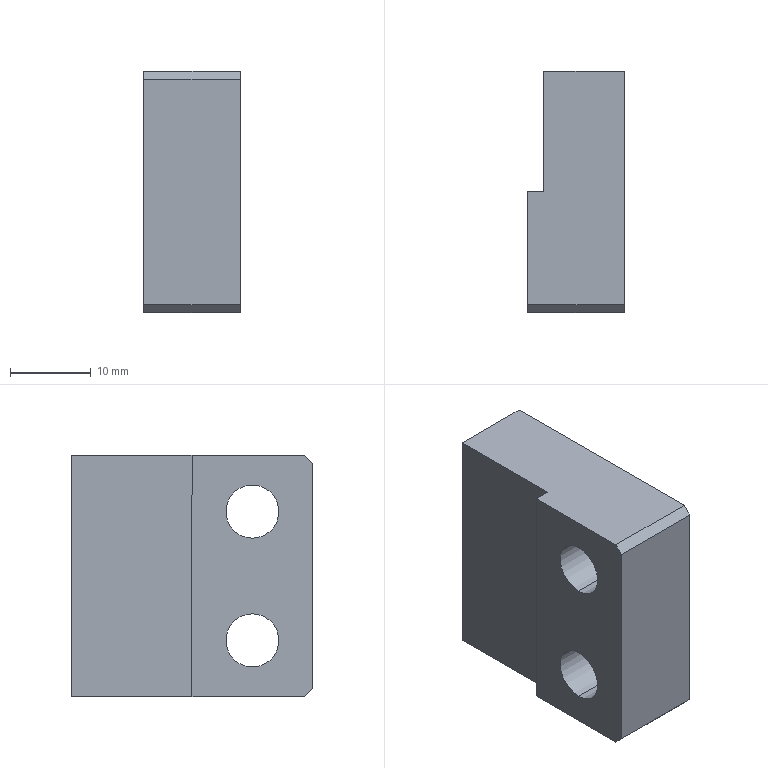Part | STEP file | M-05-006A_default | 1 solid | 20 faces | box 12 x 30 x 30 mm | volume 8337 mm3 | plane 12 | cylinder 8 | commonest cylinder face diameters 6.6 x4 11 x4
STEP:
#1=CARTESIAN_POINT('',(0.,0.,0.));
#2=DIRECTION('',(0.,0.,1.));
#3=DIRECTION('',(1.,0.,0.));
#4=AXIS2_PLACEMENT_3D('',#1,#2,#3);
#5=CARTESIAN_POINT('',(6.2,-7.5,4.7));
#6=VERTEX_POINT('',#5);
#7=CARTESIAN_POINT('',(12.2,-7.5,4.7));
#8=VERTEX_POINT('',#7);
#9=CARTESIAN_POINT('',(18.2,-7.5,4.7));
#10=DIRECTION('',(1.,0.,0.));
#11=VECTOR('',#10,1.);
#12=LINE('',#9,#11);
#13=CARTESIAN_POINT('',(18.2,-7.5,8.));
#14=DIRECTION('',(1.,0.,0.));
#15=DIRECTION('',(0.,0.,-1.));
#16=AXIS2_PLACEMENT_3D('',#13,#14,#15);
#17=CYLINDRICAL_SURFACE('',#16,3.3);
#18=CARTESIAN_POINT('',(6.283,0.));
#19=DIRECTION('',(0.,1.));
#20=VECTOR('',#19,1.);
#21=LINE('',#18,#20);
#22=(GEOMETRIC_REPRESENTATION_CONTEXT(2)PARAMETRIC_REPRESENTATION_CONTEXT()REPRESENTATION_CONTEXT('',''));
#23=DEFINITIONAL_REPRESENTATION('',(#21),#22);
#24=PCURVE('',#17,#23);
#25=CARTESIAN_POINT('',(18.2,-7.5,8.));
#26=DIRECTION('',(1.,0.,0.));
#27=DIRECTION('',(0.,0.,-1.));
#28=AXIS2_PLACEMENT_3D('',#25,#26,#27);
#29=CYLINDRICAL_SURFACE('',#28,3.3);
#30=CARTESIAN_POINT('',(0.,0.));
#31=DIRECTION('',(0.,1.));
#32=VECTOR('',#31,1.);
#33=LINE('',#30,#32);
#34=(GEOMETRIC_REPRESENTATION_CONTEXT(2)PARAMETRIC_REPRESENTATION_CONTEXT()REPRESENTATION_CONTEXT('',''));
#35=DEFINITIONAL_REPRESENTATION('',(#33),#34);
#36=PCURVE('',#29,#35);
#37=SURFACE_CURVE('',#12,(#24,#36),.PCURVE_S1.);
#38=EDGE_CURVE('',#6,#8,#37,.T.);
#39=ORIENTED_EDGE('',*,*,#38,.T.);
#40=CARTESIAN_POINT('',(12.2,-7.5,11.3));
#41=VERTEX_POINT('',#40);
#42=CARTESIAN_POINT('',(12.2,-7.5,8.));
#43=DIRECTION('',(1.,0.,0.));
#44=DIRECTION('',(0.,0.,-1.));
#45=AXIS2_PLACEMENT_3D('',#42,#43,#44);
#46=CIRCLE('',#45,3.3);
#47=CARTESIAN_POINT('',(0.,-6.));
#48=DIRECTION('',(1.,0.));
#49=VECTOR('',#48,1.);
#50=LINE('',#47,#49);
#51=(GEOMETRIC_REPRESENTATION_CONTEXT(2)PARAMETRIC_REPRESENTATION_CONTEXT()REPRESENTATION_CONTEXT('',''));
#52=DEFINITIONAL_REPRESENTATION('',(#50),#51);
#53=PCURVE('',#17,#52);
#54=CARTESIAN_POINT('',(12.2,-4.2,8.));
#55=DIRECTION('',(-1.,0.,0.));
#56=DIRECTION('',(0.,0.,1.));
#57=AXIS2_PLACEMENT_3D('',#54,#55,#56);
#58=PLANE('',#57);
#59=CARTESIAN_POINT('',(-3.3,-3.3));
#60=CARTESIAN_POINT('',(-3.3,2.416));
#61=CARTESIAN_POINT('',(1.65,-0.4421));
#62=CARTESIAN_POINT('',(6.6,-3.3));
#63=CARTESIAN_POINT('',(1.65,-6.158));
#64=CARTESIAN_POINT('',(-3.3,-9.016));
#65=CARTESIAN_POINT('',(-3.3,-3.3));
#66=(BOUNDED_CURVE()B_SPLINE_CURVE(2,(#59,#60,#61,#62,#63,#64,#65),.UNSPECIFIED.,.T.,.F.)B_SPLINE_CURVE_WITH_KNOTS((1,2,2,2,2,1),(-2.094,0.,2.094,4.189,6.283,8.378),.UNSPECIFIED.)CURVE()GEOMETRIC_REPRESENTATION_ITEM()RATIONAL_B_SPLINE_CURVE((1.,0.5,1.,0.5,1.,0.5,1.))REPRESENTATION_ITEM(''));
#67=(GEOMETRIC_REPRESENTATION_CONTEXT(2)PARAMETRIC_REPRESENTATION_CONTEXT()REPRESENTATION_CONTEXT('',''));
#68=DEFINITIONAL_REPRESENTATION('',(#66),#67);
#69=PCURVE('',#58,#68);
#70=SURFACE_CURVE('',#46,(#53,#69),.PCURVE_S1.);
#71=EDGE_CURVE('',#41,#8,#70,.T.);
#72=ORIENTED_EDGE('',*,*,#71,.F.);
#73=CARTESIAN_POINT('',(6.2,-7.5,11.3));
#74=VERTEX_POINT('',#73);
#75=CARTESIAN_POINT('',(18.2,-7.5,11.3));
#76=DIRECTION('',(1.,0.,0.));
#77=VECTOR('',#76,1.);
#78=LINE('',#75,#77);
#79=CARTESIAN_POINT('',(3.142,0.));
#80=DIRECTION('',(0.,1.));
#81=VECTOR('',#80,1.);
#82=LINE('',#79,#81);
#83=(GEOMETRIC_REPRESENTATION_CONTEXT(2)PARAMETRIC_REPRESENTATION_CONTEXT()REPRESENTATION_CONTEXT('',''));
#84=DEFINITIONAL_REPRESENTATION('',(#82),#83);
#85=PCURVE('',#17,#84);
#86=CARTESIAN_POINT('',(3.142,0.));
#87=DIRECTION('',(0.,1.));
#88=VECTOR('',#87,1.);
#89=LINE('',#86,#88);
#90=(GEOMETRIC_REPRESENTATION_CONTEXT(2)PARAMETRIC_REPRESENTATION_CONTEXT()REPRESENTATION_CONTEXT('',''));
#91=DEFINITIONAL_REPRESENTATION('',(#89),#90);
#92=PCURVE('',#29,#91);
#93=SURFACE_CURVE('',#78,(#85,#92),.PCURVE_S1.);
#94=EDGE_CURVE('',#74,#41,#93,.T.);
#95=ORIENTED_EDGE('',*,*,#94,.F.);
#96=CARTESIAN_POINT('',(6.2,-7.5,8.));
#97=DIRECTION('',(1.,0.,0.));
#98=DIRECTION('',(0.,0.,-1.));
#99=AXIS2_PLACEMENT_3D('',#96,#97,#98);
#100=CIRCLE('',#99,3.3);
#101=CARTESIAN_POINT('',(0.,-12.));
#102=DIRECTION('',(1.,0.));
#103=VECTOR('',#102,1.);
#104=LINE('',#101,#103);
#105=(GEOMETRIC_REPRESENTATION_CONTEXT(2)PARAMETRIC_REPRESENTATION_CONTEXT()REPRESENTATION_CONTEXT('',''));
#106=DEFINITIONAL_REPRESENTATION('',(#104),#105);
#107=PCURVE('',#17,#106);
#108=CARTESIAN_POINT('',(6.2,15.,15.));
#109=DIRECTION('',(1.,0.,0.));
#110=DIRECTION('',(0.,0.,-1.));
#111=AXIS2_PLACEMENT_3D('',#108,#109,#110);
#112=PLANE('',#111);
#113=CARTESIAN_POINT('',(7.,-22.5));
#114=DIRECTION('',(1.,0.));
#115=AXIS2_PLACEMENT_2D('',#113,#114);
#116=CIRCLE('',#115,3.3);
#117=(GEOMETRIC_REPRESENTATION_CONTEXT(2)PARAMETRIC_REPRESENTATION_CONTEXT()REPRESENTATION_CONTEXT('',''));
#118=DEFINITIONAL_REPRESENTATION('',(#116),#117);
#119=PCURVE('',#112,#118);
#120=SURFACE_CURVE('',#100,(#107,#119),.PCURVE_S1.);
#121=EDGE_CURVE('',#74,#6,#120,.T.);
#122=ORIENTED_EDGE('',*,*,#121,.T.);
#123=EDGE_LOOP('',(#39,#72,#95,#122));
#124=FACE_BOUND('',#123,.F.);
#125=ADVANCED_FACE('',(#124),#17,.F.);
#126=CARTESIAN_POINT('',(12.2,-7.5,2.5));
#127=VERTEX_POINT('',#126);
#128=CARTESIAN_POINT('',(18.2,-7.5,2.5));
#129=VERTEX_POINT('',#128);
#130=CARTESIAN_POINT('',(18.2,-7.5,2.5));
#131=DIRECTION('',(1.,0.,0.));
#132=VECTOR('',#131,1.);
#133=LINE('',#130,#132);
#134=CARTESIAN_POINT('',(18.2,-7.5,8.));
#135=DIRECTION('',(1.,0.,0.));
#136=DIRECTION('',(0.,0.,-1.));
#137=AXIS2_PLACEMENT_3D('',#134,#135,#136);
#138=CYLINDRICAL_SURFACE('',#137,5.5);
#139=CARTESIAN_POINT('',(6.283,0.));
#140=DIRECTION('',(0.,1.));
#141=VECTOR('',#140,1.);
#142=LINE('',#139,#141);
#143=(GEOMETRIC_REPRESENTATION_CONTEXT(2)PARAMETRIC_REPRESENTATION_CONTEXT()REPRESENTATION_CONTEXT('',''));
#144=DEFINITIONAL_REPRESENTATION('',(#142),#143);
#145=PCURVE('',#138,#144);
#146=CARTESIAN_POINT('',(18.2,-7.5,8.));
#147=DIRECTION('',(1.,0.,0.));
#148=DIRECTION('',(0.,0.,-1.));
#149=AXIS2_PLACEMENT_3D('',#146,#147,#148);
#150=CYLINDRICAL_SURFACE('',#149,5.5);
#151=CARTESIAN_POINT('',(0.,0.));
#152=DIRECTION('',(0.,1.));
#153=VECTOR('',#152,1.);
#154=LINE('',#151,#153);
#155=(GEOMETRIC_REPRESENTATION_CONTEXT(2)PARAMETRIC_REPRESENTATION_CONTEXT()REPRESENTATION_CONTEXT('',''));
#156=DEFINITIONAL_REPRESENTATION('',(#154),#155);
#157=PCURVE('',#150,#156);
#158=SURFACE_CURVE('',#133,(#145,#157),.PCURVE_S1.);
#159=EDGE_CURVE('',#127,#129,#158,.T.);
#160=ORIENTED_EDGE('',*,*,#159,.T.);
#161=CARTESIAN_POINT('',(18.2,-7.5,13.5));
#162=VERTEX_POINT('',#161);
#163=CARTESIAN_POINT('',(18.2,-7.5,8.));
#164=DIRECTION('',(1.,0.,0.));
#165=DIRECTION('',(0.,0.,-1.));
#166=AXIS2_PLACEMENT_3D('',#163,#164,#165);
#167=CIRCLE('',#166,5.5);
#168=CARTESIAN_POINT('',(0.,0.));
#169=DIRECTION('',(1.,0.));
#170=VECTOR('',#169,1.);
#171=LINE('',#168,#170);
#172=(GEOMETRIC_REPRESENTATION_CONTEXT(2)PARAMETRIC_REPRESENTATION_CONTEXT()REPRESENTATION_CONTEXT('',''));
#173=DEFINITIONAL_REPRESENTATION('',(#171),#172);
#174=PCURVE('',#138,#173);
#175=CARTESIAN_POINT('',(18.2,15.,15.));
#176=DIRECTION('',(-1.,0.,0.));
#177=DIRECTION('',(0.,0.,1.));
#178=AXIS2_PLACEMENT_3D('',#175,#176,#177);
#179=PLANE('',#178);
#180=CARTESIAN_POINT('',(-12.5,-22.5));
#181=CARTESIAN_POINT('',(-12.5,-12.974));
#182=CARTESIAN_POINT('',(-4.25,-17.737));
#183=CARTESIAN_POINT('',(4.,-22.5));
#184=CARTESIAN_POINT('',(-4.25,-27.263));
#185=CARTESIAN_POINT('',(-12.5,-32.026));
#186=CARTESIAN_POINT('',(-12.5,-22.5));
#187=(BOUNDED_CURVE()B_SPLINE_CURVE(2,(#180,#181,#182,#183,#184,#185,#186),.UNSPECIFIED.,.T.,.F.)B_SPLINE_CURVE_WITH_KNOTS((1,2,2,2,2,1),(-2.094,0.,2.094,4.189,6.283,8.378),.UNSPECIFIED.)CURVE()GEOMETRIC_REPRESENTATION_ITEM()RATIONAL_B_SPLINE_CURVE((1.,0.5,1.,0.5,1.,0.5,1.))REPRESENTATION_ITEM(''));
#188=(GEOMETRIC_REPRESENTATION_CONTEXT(2)PARAMETRIC_REPRESENTATION_CONTEXT()REPRESENTATION_CONTEXT('',''));
#189=DEFINITIONAL_REPRESENTATION('',(#187),#188);
#190=PCURVE('',#179,#189);
#191=SURFACE_CURVE('',#167,(#174,#190),.PCURVE_S1.);
#192=EDGE_CURVE('',#162,#129,#191,.T.);
#193=ORIENTED_EDGE('',*,*,#192,.F.);
#194=CARTESIAN_POINT('',(12.2,-7.5,13.5));
#195=VERTEX_POINT('',#194);
#196=CARTESIAN_POINT('',(18.2,-7.5,13.5));
#197=DIRECTION('',(1.,0.,0.));
#198=VECTOR('',#197,1.);
#199=LINE('',#196,#198);
#200=CARTESIAN_POINT('',(3.142,0.));
#201=DIRECTION('',(0.,1.));
#202=VECTOR('',#201,1.);
#203=LINE('',#200,#202);
#204=(GEOMETRIC_REPRESENTATION_CONTEXT(2)PARAMETRIC_REPRESENTATION_CONTEXT()REPRESENTATION_CONTEXT('',''));
#205=DEFINITIONAL_REPRESENTATION('',(#203),#204);
#206=PCURVE('',#138,#205);
#207=CARTESIAN_POINT('',(3.142,0.));
#208=DIRECTION('',(0.,1.));
#209=VECTOR('',#208,1.);
#210=LINE('',#207,#209);
#211=(GEOMETRIC_REPRESENTATION_CONTEXT(2)PARAMETRIC_REPRESENTATION_CONTEXT()REPRESENTATION_CONTEXT('',''));
#212=DEFINITIONAL_REPRESENTATION('',(#210),#211);
#213=PCURVE('',#150,#212);
#214=SURFACE_CURVE('',#199,(#206,#213),.PCURVE_S1.);
#215=EDGE_CURVE('',#195,#162,#214,.T.);
#216=ORIENTED_EDGE('',*,*,#215,.F.);
#217=CARTESIAN_POINT('',(12.2,-7.5,8.));
#218=DIRECTION('',(1.,0.,0.));
#219=DIRECTION('',(0.,0.,-1.));
#220=AXIS2_PLACEMENT_3D('',#217,#218,#219);
#221=CIRCLE('',#220,5.5);
#222=CARTESIAN_POINT('',(0.,-6.));
#223=DIRECTION('',(1.,0.));
#224=VECTOR('',#223,1.);
#225=LINE('',#222,#224);
#226=(GEOMETRIC_REPRESENTATION_CONTEXT(2)PARAMETRIC_REPRESENTATION_CONTEXT()REPRESENTATION_CONTEXT('',''));
#227=DEFINITIONAL_REPRESENTATION('',(#225),#226);
#228=PCURVE('',#138,#227);
#229=CARTESIAN_POINT('',(-5.5,-3.3));
#230=CARTESIAN_POINT('',(-5.5,6.226));
#231=CARTESIAN_POINT('',(2.75,1.463));
#232=CARTESIAN_POINT('',(11.,-3.3));
#233=CARTESIAN_POINT('',(2.75,-8.063));
#234=CARTESIAN_POINT('',(-5.5,-12.826));
#235=CARTESIAN_POINT('',(-5.5,-3.3));
#236=(BOUNDED_CURVE()B_SPLINE_CURVE(2,(#229,#230,#231,#232,#233,#234,#235),.UNSPECIFIED.,.T.,.F.)B_SPLINE_CURVE_WITH_KNOTS((1,2,2,2,2,1),(-2.094,0.,2.094,4.189,6.283,8.378),.UNSPECIFIED.)CURVE()GEOMETRIC_REPRESENTATION_ITEM()RATIONAL_B_SPLINE_CURVE((1.,0.5,1.,0.5,1.,0.5,1.))REPRESENTATION_ITEM(''));
#237=(GEOMETRIC_REPRESENTATION_CONTEXT(2)PARAMETRIC_REPRESENTATION_CONTEXT()REPRESENTATION_CONTEXT('',''));
#238=DEFINITIONAL_REPRESENTATION('',(#236),#237);
#239=PCURVE('',#58,#238);
#240=SURFACE_CURVE('',#221,(#228,#239),.PCURVE_S1.);
#241=EDGE_CURVE('',#195,#127,#240,.T.);
#242=ORIENTED_EDGE('',*,*,#241,.T.);
#243=EDGE_LOOP('',(#160,#193,#216,#242));
#244=FACE_BOUND('',#243,.F.);
#245=ADVANCED_FACE('',(#244),#138,.F.);
#246=CARTESIAN_POINT('',(6.2,-7.5,-11.3));
#247=VERTEX_POINT('',#246);
#248=CARTESIAN_POINT('',(12.2,-7.5,-11.3));
#249=VERTEX_POINT('',#248);
#250=CARTESIAN_POINT('',(18.2,-7.5,-11.3));
#251=DIRECTION('',(1.,0.,0.));
#252=VECTOR('',#251,1.);
#253=LINE('',#250,#252);
#254=CARTESIAN_POINT('',(18.2,-7.5,-8.));
#255=DIRECTION('',(1.,0.,0.));
#256=DIRECTION('',(0.,0.,-1.));
#257=AXIS2_PLACEMENT_3D('',#254,#255,#256);
#258=CYLINDRICAL_SURFACE('',#257,3.3);
#259=CARTESIAN_POINT('',(6.283,0.));
#260=DIRECTION('',(0.,1.));
#261=VECTOR('',#260,1.);
#262=LINE('',#259,#261);
#263=(GEOMETRIC_REPRESENTATION_CONTEXT(2)PARAMETRIC_REPRESENTATION_CONTEXT()REPRESENTATION_CONTEXT('',''));
#264=DEFINITIONAL_REPRESENTATION('',(#262),#263);
#265=PCURVE('',#258,#264);
#266=CARTESIAN_POINT('',(18.2,-7.5,-8.));
#267=DIRECTION('',(1.,0.,0.));
#268=DIRECTION('',(0.,0.,-1.));
#269=AXIS2_PLACEMENT_3D('',#266,#267,#268);
#270=CYLINDRICAL_SURFACE('',#269,3.3);
#271=CARTESIAN_POINT('',(0.,0.));
#272=DIRECTION('',(0.,1.));
#273=VECTOR('',#272,1.);
#274=LINE('',#271,#273);
#275=(GEOMETRIC_REPRESENTATION_CONTEXT(2)PARAMETRIC_REPRESENTATION_CONTEXT()REPRESENTATION_CONTEXT('',''));
#276=DEFINITIONAL_REPRESENTATION('',(#274),#275);
#277=PCURVE('',#270,#276);
#278=SURFACE_CURVE('',#253,(#265,#277),.PCURVE_S1.);
#279=EDGE_CURVE('',#247,#249,#278,.T.);
#280=ORIENTED_EDGE('',*,*,#279,.T.);
#281=CARTESIAN_POINT('',(12.2,-7.5,-4.7));
#282=VERTEX_POINT('',#281);
#283=CARTESIAN_POINT('',(12.2,-7.5,-8.));
#284=DIRECTION('',(1.,0.,0.));
#285=DIRECTION('',(0.,0.,-1.));
#286=AXIS2_PLACEMENT_3D('',#283,#284,#285);
#287=CIRCLE('',#286,3.3);
#288=CARTESIAN_POINT('',(0.,-6.));
#289=DIRECTION('',(1.,0.));
#290=VECTOR('',#289,1.);
#291=LINE('',#288,#290);
#292=(GEOMETRIC_REPRESENTATION_CONTEXT(2)PARAMETRIC_REPRESENTATION_CONTEXT()REPRESENTATION_CONTEXT('',''));
#293=DEFINITIONAL_REPRESENTATION('',(#291),#292);
#294=PCURVE('',#258,#293);
#295=CARTESIAN_POINT('',(12.2,-4.2,-8.));
#296=DIRECTION('',(-1.,0.,0.));
#297=DIRECTION('',(0.,0.,1.));
#298=AXIS2_PLACEMENT_3D('',#295,#296,#297);
#299=PLANE('',#298);
#300=CARTESIAN_POINT('',(-3.3,-3.3));
#301=CARTESIAN_POINT('',(-3.3,2.416));
#302=CARTESIAN_POINT('',(1.65,-0.4421));
#303=CARTESIAN_POINT('',(6.6,-3.3));
#304=CARTESIAN_POINT('',(1.65,-6.158));
#305=CARTESIAN_POINT('',(-3.3,-9.016));
#306=CARTESIAN_POINT('',(-3.3,-3.3));
#307=(BOUNDED_CURVE()B_SPLINE_CURVE(2,(#300,#301,#302,#303,#304,#305,#306),.UNSPECIFIED.,.T.,.F.)B_SPLINE_CURVE_WITH_KNOTS((1,2,2,2,2,1),(-2.094,0.,2.094,4.189,6.283,8.378),.UNSPECIFIED.)CURVE()GEOMETRIC_REPRESENTATION_ITEM()RATIONAL_B_SPLINE_CURVE((1.,0.5,1.,0.5,1.,0.5,1.))REPRESENTATION_ITEM(''));
#308=(GEOMETRIC_REPRESENTATION_CONTEXT(2)PARAMETRIC_REPRESENTATION_CONTEXT()REPRESENTATION_CONTEXT('',''));
#309=DEFINITIONAL_REPRESENTATION('',(#307),#308);
#310=PCURVE('',#299,#309);
#311=SURFACE_CURVE('',#287,(#294,#310),.PCURVE_S1.);
#312=EDGE_CURVE('',#282,#249,#311,.T.);
#313=ORIENTED_EDGE('',*,*,#312,.F.);
#314=CARTESIAN_POINT('',(6.2,-7.5,-4.7));
#315=VERTEX_POINT('',#314);
#316=CARTESIAN_POINT('',(18.2,-7.5,-4.7));
#317=DIRECTION('',(1.,0.,0.));
#318=VECTOR('',#317,1.);
#319=LINE('',#316,#318);
#320=CARTESIAN_POINT('',(3.142,0.));
#321=DIRECTION('',(0.,1.));
#322=VECTOR('',#321,1.);
#323=LINE('',#320,#322);
#324=(GEOMETRIC_REPRESENTATION_CONTEXT(2)PARAMETRIC_REPRESENTATION_CONTEXT()REPRESENTATION_CONTEXT('',''));
#325=DEFINITIONAL_REPRESENTATION('',(#323),#324);
#326=PCURVE('',#258,#325);
#327=CARTESIAN_POINT('',(3.142,0.));
#328=DIRECTION('',(0.,1.));
#329=VECTOR('',#328,1.);
#330=LINE('',#327,#329);
#331=(GEOMETRIC_REPRESENTATION_CONTEXT(2)PARAMETRIC_REPRESENTATION_CONTEXT()REPRESENTATION_CONTEXT('',''));
#332=DEFINITIONAL_REPRESENTATION('',(#330),#331);
#333=PCURVE('',#270,#332);
#334=SURFACE_CURVE('',#319,(#326,#333),.PCURVE_S1.);
#335=EDGE_CURVE('',#315,#282,#334,.T.);
#336=ORIENTED_EDGE('',*,*,#335,.F.);
#337=CARTESIAN_POINT('',(6.2,-7.5,-8.));
#338=DIRECTION('',(1.,0.,0.));
#339=DIRECTION('',(0.,0.,-1.));
#340=AXIS2_PLACEMENT_3D('',#337,#338,#339);
#341=CIRCLE('',#340,3.3);
#342=CARTESIAN_POINT('',(0.,-12.));
#343=DIRECTION('',(1.,0.));
#344=VECTOR('',#343,1.);
#345=LINE('',#342,#344);
#346=(GEOMETRIC_REPRESENTATION_CONTEXT(2)PARAMETRIC_REPRESENTATION_CONTEXT()REPRESENTATION_CONTEXT('',''));
#347=DEFINITIONAL_REPRESENTATION('',(#345),#346);
#348=PCURVE('',#258,#347);
#349=CARTESIAN_POINT('',(23.,-22.5));
#350=DIRECTION('',(1.,0.));
#351=AXIS2_PLACEMENT_2D('',#349,#350);
#352=CIRCLE('',#351,3.3);
#353=(GEOMETRIC_REPRESENTATION_CONTEXT(2)PARAMETRIC_REPRESENTATION_CONTEXT()REPRESENTATION_CONTEXT('',''));
#354=DEFINITIONAL_REPRESENTATION('',(#352),#353);
#355=PCURVE('',#112,#354);
#356=SURFACE_CURVE('',#341,(#348,#355),.PCURVE_S1.);
#357=EDGE_CURVE('',#315,#247,#356,.T.);
#358=ORIENTED_EDGE('',*,*,#357,.T.);
#359=EDGE_LOOP('',(#280,#313,#336,#358));
#360=FACE_BOUND('',#359,.F.);
#361=ADVANCED_FACE('',(#360),#258,.F.);
#362=CARTESIAN_POINT('',(12.2,-7.5,-13.5));
#363=VERTEX_POINT('',#362);
#364=CARTESIAN_POINT('',(18.2,-7.5,-13.5));
#365=VERTEX_POINT('',#364);
#366=CARTESIAN_POINT('',(18.2,-7.5,-13.5));
#367=DIRECTION('',(1.,0.,0.));
#368=VECTOR('',#367,1.);
#369=LINE('',#366,#368);
#370=CARTESIAN_POINT('',(18.2,-7.5,-8.));
#371=DIRECTION('',(1.,0.,0.));
#372=DIRECTION('',(0.,0.,-1.));
#373=AXIS2_PLACEMENT_3D('',#370,#371,#372);
#374=CYLINDRICAL_SURFACE('',#373,5.5);
#375=CARTESIAN_POINT('',(6.283,0.));
#376=DIRECTION('',(0.,1.));
#377=VECTOR('',#376,1.);
#378=LINE('',#375,#377);
#379=(GEOMETRIC_REPRESENTATION_CONTEXT(2)PARAMETRIC_REPRESENTATION_CONTEXT()REPRESENTATION_CONTEXT('',''));
#380=DEFINITIONAL_REPRESENTATION('',(#378),#379);
#381=PCURVE('',#374,#380);
#382=CARTESIAN_POINT('',(18.2,-7.5,-8.));
#383=DIRECTION('',(1.,0.,0.));
#384=DIRECTION('',(0.,0.,-1.));
#385=AXIS2_PLACEMENT_3D('',#382,#383,#384);
#386=CYLINDRICAL_SURFACE('',#385,5.5);
#387=CARTESIAN_POINT('',(0.,0.));
#388=DIRECTION('',(0.,1.));
#389=VECTOR('',#388,1.);
#390=LINE('',#387,#389);
#391=(GEOMETRIC_REPRESENTATION_CONTEXT(2)PARAMETRIC_REPRESENTATION_CONTEXT()REPRESENTATION_CONTEXT('',''));
#392=DEFINITIONAL_REPRESENTATION('',(#390),#391);
#393=PCURVE('',#386,#392);
#394=SURFACE_CURVE('',#369,(#381,#393),.PCURVE_S1.);
#395=EDGE_CURVE('',#363,#365,#394,.T.);
#396=ORIENTED_EDGE('',*,*,#395,.T.);
#397=CARTESIAN_POINT('',(18.2,-7.5,-2.5));
#398=VERTEX_POINT('',#397);
#399=CARTESIAN_POINT('',(18.2,-7.5,-8.));
#400=DIRECTION('',(1.,0.,0.));
#401=DIRECTION('',(0.,0.,-1.));
#402=AXIS2_PLACEMENT_3D('',#399,#400,#401);
#403=CIRCLE('',#402,5.5);
#404=CARTESIAN_POINT('',(0.,0.));
#405=DIRECTION('',(1.,0.));
#406=VECTOR('',#405,1.);
#407=LINE('',#404,#406);
#408=(GEOMETRIC_REPRESENTATION_CONTEXT(2)PARAMETRIC_REPRESENTATION_CONTEXT()REPRESENTATION_CONTEXT('',''));
#409=DEFINITIONAL_REPRESENTATION('',(#407),#408);
#410=PCURVE('',#374,#409);
#411=CARTESIAN_POINT('',(-28.5,-22.5));
#412=CARTESIAN_POINT('',(-28.5,-12.974));
#413=CARTESIAN_POINT('',(-20.25,-17.737));
#414=CARTESIAN_POINT('',(-12.,-22.5));
#415=CARTESIAN_POINT('',(-20.25,-27.263));
#416=CARTESIAN_POINT('',(-28.5,-32.026));
#417=CARTESIAN_POINT('',(-28.5,-22.5));
#418=(BOUNDED_CURVE()B_SPLINE_CURVE(2,(#411,#412,#413,#414,#415,#416,#417),.UNSPECIFIED.,.T.,.F.)B_SPLINE_CURVE_WITH_KNOTS((1,2,2,2,2,1),(-2.094,0.,2.094,4.189,6.283,8.378),.UNSPECIFIED.)CURVE()GEOMETRIC_REPRESENTATION_ITEM()RATIONAL_B_SPLINE_CURVE((1.,0.5,1.,0.5,1.,0.5,1.))REPRESENTATION_ITEM(''));
#419=(GEOMETRIC_REPRESENTATION_CONTEXT(2)PARAMETRIC_REPRESENTATION_CONTEXT()REPRESENTATION_CONTEXT('',''));
#420=DEFINITIONAL_REPRESENTATION('',(#418),#419);
#421=PCURVE('',#179,#420);
#422=SURFACE_CURVE('',#403,(#410,#421),.PCURVE_S1.);
#423=EDGE_CURVE('',#398,#365,#422,.T.);
#424=ORIENTED_EDGE('',*,*,#423,.F.);
#425=CARTESIAN_POINT('',(12.2,-7.5,-2.5));
#426=VERTEX_POINT('',#425);
#427=CARTESIAN_POINT('',(18.2,-7.5,-2.5));
#428=DIRECTION('',(1.,0.,0.));
#429=VECTOR('',#428,1.);
#430=LINE('',#427,#429);
#431=CARTESIAN_POINT('',(3.142,0.));
#432=DIRECTION('',(0.,1.));
#433=VECTOR('',#432,1.);
#434=LINE('',#431,#433);
#435=(GEOMETRIC_REPRESENTATION_CONTEXT(2)PARAMETRIC_REPRESENTATION_CONTEXT()REPRESENTATION_CONTEXT('',''));
#436=DEFINITIONAL_REPRESENTATION('',(#434),#435);
#437=PCURVE('',#374,#436);
#438=CARTESIAN_POINT('',(3.142,0.));
#439=DIRECTION('',(0.,1.));
#440=VECTOR('',#439,1.);
#441=LINE('',#438,#440);
#442=(GEOMETRIC_REPRESENTATION_CONTEXT(2)PARAMETRIC_REPRESENTATION_CONTEXT()REPRESENTATION_CONTEXT('',''));
#443=DEFINITIONAL_REPRESENTATION('',(#441),#442);
#444=PCURVE('',#386,#443);
#445=SURFACE_CURVE('',#430,(#437,#444),.PCURVE_S1.);
#446=EDGE_CURVE('',#426,#398,#445,.T.);
#447=ORIENTED_EDGE('',*,*,#446,.F.);
#448=CARTESIAN_POINT('',(12.2,-7.5,-8.));
#449=DIRECTION('',(1.,0.,0.));
#450=DIRECTION('',(0.,0.,-1.));
#451=AXIS2_PLACEMENT_3D('',#448,#449,#450);
#452=CIRCLE('',#451,5.5);
#453=CARTESIAN_POINT('',(0.,-6.));
#454=DIRECTION('',(1.,0.));
#455=VECTOR('',#454,1.);
#456=LINE('',#453,#455);
#457=(GEOMETRIC_REPRESENTATION_CONTEXT(2)PARAMETRIC_REPRESENTATION_CONTEXT()REPRESENTATION_CONTEXT('',''));
#458=DEFINITIONAL_REPRESENTATION('',(#456),#457);
#459=PCURVE('',#374,#458);
#460=CARTESIAN_POINT('',(-5.5,-3.3));
#461=CARTESIAN_POINT('',(-5.5,6.226));
#462=CARTESIAN_POINT('',(2.75,1.463));
#463=CARTESIAN_POINT('',(11.,-3.3));
#464=CARTESIAN_POINT('',(2.75,-8.063));
#465=CARTESIAN_POINT('',(-5.5,-12.826));
#466=CARTESIAN_POINT('',(-5.5,-3.3));
#467=(BOUNDED_CURVE()B_SPLINE_CURVE(2,(#460,#461,#462,#463,#464,#465,#466),.UNSPECIFIED.,.T.,.F.)B_SPLINE_CURVE_WITH_KNOTS((1,2,2,2,2,1),(-2.094,0.,2.094,4.189,6.283,8.378),.UNSPECIFIED.)CURVE()GEOMETRIC_REPRESENTATION_ITEM()RATIONAL_B_SPLINE_CURVE((1.,0.5,1.,0.5,1.,0.5,1.))REPRESENTATION_ITEM(''));
#468=(GEOMETRIC_REPRESENTATION_CONTEXT(2)PARAMETRIC_REPRESENTATION_CONTEXT()REPRESENTATION_CONTEXT('',''));
#469=DEFINITIONAL_REPRESENTATION('',(#467),#468);
#470=PCURVE('',#299,#469);
#471=SURFACE_CURVE('',#452,(#459,#470),.PCURVE_S1.);
#472=EDGE_CURVE('',#426,#363,#471,.T.);
#473=ORIENTED_EDGE('',*,*,#472,.T.);
#474=EDGE_LOOP('',(#396,#424,#447,#473));
#475=FACE_BOUND('',#474,.F.);
#476=ADVANCED_FACE('',(#475),#374,.F.);
#477=CARTESIAN_POINT('',(8.2,15.,15.));
#478=VERTEX_POINT('',#477);
#479=CARTESIAN_POINT('',(8.2,15.,-15.));
#480=VERTEX_POINT('',#479);
#481=CARTESIAN_POINT('',(8.2,15.,-15.));
#482=DIRECTION('',(0.,0.,-1.));
#483=VECTOR('',#482,1.);
#484=LINE('',#481,#483);
#485=CARTESIAN_POINT('',(6.2,15.,15.));
#486=DIRECTION('',(0.,-1.,0.));
#487=DIRECTION('',(0.,0.,-1.));
#488=AXIS2_PLACEMENT_3D('',#485,#486,#487);
#489=PLANE('',#488);
#490=CARTESIAN_POINT('',(30.,2.));
#491=DIRECTION('',(1.,0.));
#492=VECTOR('',#491,1.);
#493=LINE('',#490,#492);
#494=(GEOMETRIC_REPRESENTATION_CONTEXT(2)PARAMETRIC_REPRESENTATION_CONTEXT()REPRESENTATION_CONTEXT('',''));
#495=DEFINITIONAL_REPRESENTATION('',(#493),#494);
#496=PCURVE('',#489,#495);
#497=CARTESIAN_POINT('',(8.2,0.,-15.));
#498=DIRECTION('',(-1.,0.,0.));
#499=DIRECTION('',(0.,0.,1.));
#500=AXIS2_PLACEMENT_3D('',#497,#498,#499);
#501=PLANE('',#500);
#502=CARTESIAN_POINT('',(0.,15.));
#503=DIRECTION('',(-1.,0.));
#504=VECTOR('',#503,1.);
#505=LINE('',#502,#504);
#506=(GEOMETRIC_REPRESENTATION_CONTEXT(2)PARAMETRIC_REPRESENTATION_CONTEXT()REPRESENTATION_CONTEXT('',''));
#507=DEFINITIONAL_REPRESENTATION('',(#505),#506);
#508=PCURVE('',#501,#507);
#509=SURFACE_CURVE('',#484,(#496,#508),.PCURVE_S1.);
#510=EDGE_CURVE('',#478,#480,#509,.T.);
#511=ORIENTED_EDGE('',*,*,#510,.F.);
#512=CARTESIAN_POINT('',(18.2,15.,15.));
#513=VERTEX_POINT('',#512);
#514=CARTESIAN_POINT('',(6.2,15.,15.));
#515=DIRECTION('',(-1.,0.,0.));
#516=VECTOR('',#515,1.);
#517=LINE('',#514,#516);
#518=CARTESIAN_POINT('',(0.,0.));
#519=DIRECTION('',(0.,-1.));
#520=VECTOR('',#519,1.);
#521=LINE('',#518,#520);
#522=(GEOMETRIC_REPRESENTATION_CONTEXT(2)PARAMETRIC_REPRESENTATION_CONTEXT()REPRESENTATION_CONTEXT('',''));
#523=DEFINITIONAL_REPRESENTATION('',(#521),#522);
#524=PCURVE('',#489,#523);
#525=CARTESIAN_POINT('',(18.2,-15.,15.));
#526=DIRECTION('',(0.,0.,-1.));
#527=DIRECTION('',(-1.,0.,0.));
#528=AXIS2_PLACEMENT_3D('',#525,#526,#527);
#529=PLANE('',#528);
#530=CARTESIAN_POINT('',(12.,30.));
#531=DIRECTION('',(1.,0.));
#532=VECTOR('',#531,1.);
#533=LINE('',#530,#532);
#534=(GEOMETRIC_REPRESENTATION_CONTEXT(2)PARAMETRIC_REPRESENTATION_CONTEXT()REPRESENTATION_CONTEXT('',''));
#535=DEFINITIONAL_REPRESENTATION('',(#533),#534);
#536=PCURVE('',#529,#535);
#537=SURFACE_CURVE('',#517,(#524,#536),.PCURVE_S1.);
#538=EDGE_CURVE('',#513,#478,#537,.T.);
#539=ORIENTED_EDGE('',*,*,#538,.F.);
#540=CARTESIAN_POINT('',(18.2,15.,-15.));
#541=VERTEX_POINT('',#540);
#542=CARTESIAN_POINT('',(18.2,15.,15.));
#543=DIRECTION('',(0.,0.,-1.));
#544=VECTOR('',#543,1.);
#545=LINE('',#542,#544);
#546=CARTESIAN_POINT('',(0.,12.));
#547=DIRECTION('',(1.,0.));
#548=VECTOR('',#547,1.);
#549=LINE('',#546,#548);
#550=(GEOMETRIC_REPRESENTATION_CONTEXT(2)PARAMETRIC_REPRESENTATION_CONTEXT()REPRESENTATION_CONTEXT('',''));
#551=DEFINITIONAL_REPRESENTATION('',(#549),#550);
#552=PCURVE('',#489,#551);
#553=CARTESIAN_POINT('',(0.,0.));
#554=DIRECTION('',(-1.,0.));
#555=VECTOR('',#554,1.);
#556=LINE('',#553,#555);
#557=(GEOMETRIC_REPRESENTATION_CONTEXT(2)PARAMETRIC_REPRESENTATION_CONTEXT()REPRESENTATION_CONTEXT('',''));
#558=DEFINITIONAL_REPRESENTATION('',(#556),#557);
#559=PCURVE('',#179,#558);
#560=SURFACE_CURVE('',#545,(#552,#559),.PCURVE_S1.);
#561=EDGE_CURVE('',#513,#541,#560,.T.);
#562=ORIENTED_EDGE('',*,*,#561,.T.);
#563=CARTESIAN_POINT('',(6.2,15.,-15.));
#564=DIRECTION('',(-1.,0.,0.));
#565=VECTOR('',#564,1.);
#566=LINE('',#563,#565);
#567=CARTESIAN_POINT('',(30.,0.));
#568=DIRECTION('',(0.,-1.));
#569=VECTOR('',#568,1.);
#570=LINE('',#567,#569);
#571=(GEOMETRIC_REPRESENTATION_CONTEXT(2)PARAMETRIC_REPRESENTATION_CONTEXT()REPRESENTATION_CONTEXT('',''));
#572=DEFINITIONAL_REPRESENTATION('',(#570),#571);
#573=PCURVE('',#489,#572);
#574=CARTESIAN_POINT('',(18.2,-15.,-15.));
#575=DIRECTION('',(0.,0.,-1.));
#576=DIRECTION('',(-1.,0.,0.));
#577=AXIS2_PLACEMENT_3D('',#574,#575,#576);
#578=PLANE('',#577);
#579=CARTESIAN_POINT('',(12.,30.));
#580=DIRECTION('',(1.,0.));
#581=VECTOR('',#580,1.);
#582=LINE('',#579,#581);
#583=(GEOMETRIC_REPRESENTATION_CONTEXT(2)PARAMETRIC_REPRESENTATION_CONTEXT()REPRESENTATION_CONTEXT('',''));
#584=DEFINITIONAL_REPRESENTATION('',(#582),#583);
#585=PCURVE('',#578,#584);
#586=SURFACE_CURVE('',#566,(#573,#585),.PCURVE_S1.);
#587=EDGE_CURVE('',#541,#480,#586,.T.);
#588=ORIENTED_EDGE('',*,*,#587,.T.);
#589=EDGE_LOOP('',(#511,#539,#562,#588));
#590=FACE_BOUND('',#589,.T.);
#591=ADVANCED_FACE('',(#590),#489,.F.);
#592=CARTESIAN_POINT('',(18.2,-15.,14.));
#593=VERTEX_POINT('',#592);
#594=CARTESIAN_POINT('',(18.2,-15.,-14.));
#595=VERTEX_POINT('',#594);
#596=CARTESIAN_POINT('',(18.2,-15.,15.));
#597=DIRECTION('',(0.,0.,-1.));
#598=VECTOR('',#597,1.);
#599=LINE('',#596,#598);
#600=CARTESIAN_POINT('',(6.2,-15.,15.));
#601=DIRECTION('',(0.,1.,0.));
#602=DIRECTION('',(0.,0.,1.));
#603=AXIS2_PLACEMENT_3D('',#600,#601,#602);
#604=PLANE('',#603);
#605=CARTESIAN_POINT('',(0.,12.));
#606=DIRECTION('',(-1.,0.));
#607=VECTOR('',#606,1.);
#608=LINE('',#605,#607);
#609=(GEOMETRIC_REPRESENTATION_CONTEXT(2)PARAMETRIC_REPRESENTATION_CONTEXT()REPRESENTATION_CONTEXT('',''));
#610=DEFINITIONAL_REPRESENTATION('',(#608),#609);
#611=PCURVE('',#604,#610);
#612=CARTESIAN_POINT('',(0.,-30.));
#613=DIRECTION('',(-1.,0.));
#614=VECTOR('',#613,1.);
#615=LINE('',#612,#614);
#616=(GEOMETRIC_REPRESENTATION_CONTEXT(2)PARAMETRIC_REPRESENTATION_CONTEXT()REPRESENTATION_CONTEXT('',''));
#617=DEFINITIONAL_REPRESENTATION('',(#615),#616);
#618=PCURVE('',#179,#617);
#619=SURFACE_CURVE('',#599,(#611,#618),.PCURVE_S1.);
#620=EDGE_CURVE('',#593,#595,#619,.T.);
#621=ORIENTED_EDGE('',*,*,#620,.F.);
#622=CARTESIAN_POINT('',(6.2,-15.,14.));
#623=VERTEX_POINT('',#622);
#624=CARTESIAN_POINT('',(6.2,-15.,14.));
#625=DIRECTION('',(-1.,0.,0.));
#626=VECTOR('',#625,1.);
#627=LINE('',#624,#626);
#628=CARTESIAN_POINT('',(-1.,0.));
#629=DIRECTION('',(0.,-1.));
#630=VECTOR('',#629,1.);
#631=LINE('',#628,#630);
#632=(GEOMETRIC_REPRESENTATION_CONTEXT(2)PARAMETRIC_REPRESENTATION_CONTEXT()REPRESENTATION_CONTEXT('',''));
#633=DEFINITIONAL_REPRESENTATION('',(#631),#632);
#634=PCURVE('',#604,#633);
#635=CARTESIAN_POINT('',(18.2,-14.,15.));
#636=DIRECTION('',(0.,0.7071,-0.7071));
#637=DIRECTION('',(0.,0.7071,0.7071));
#638=AXIS2_PLACEMENT_3D('',#635,#636,#637);
#639=PLANE('',#638);
#640=CARTESIAN_POINT('',(-1.414,-12.));
#641=DIRECTION('',(0.,-1.));
#642=VECTOR('',#641,1.);
#643=LINE('',#640,#642);
#644=(GEOMETRIC_REPRESENTATION_CONTEXT(2)PARAMETRIC_REPRESENTATION_CONTEXT()REPRESENTATION_CONTEXT('',''));
#645=DEFINITIONAL_REPRESENTATION('',(#643),#644);
#646=PCURVE('',#639,#645);
#647=SURFACE_CURVE('',#627,(#634,#646),.PCURVE_S1.);
#648=EDGE_CURVE('',#593,#623,#647,.T.);
#649=ORIENTED_EDGE('',*,*,#648,.T.);
#650=CARTESIAN_POINT('',(6.2,-15.,-14.));
#651=VERTEX_POINT('',#650);
#652=CARTESIAN_POINT('',(6.2,-15.,15.));
#653=DIRECTION('',(0.,0.,-1.));
#654=VECTOR('',#653,1.);
#655=LINE('',#652,#654);
#656=CARTESIAN_POINT('',(0.,0.));
#657=DIRECTION('',(-1.,0.));
#658=VECTOR('',#657,1.);
#659=LINE('',#656,#658);
#660=(GEOMETRIC_REPRESENTATION_CONTEXT(2)PARAMETRIC_REPRESENTATION_CONTEXT()REPRESENTATION_CONTEXT('',''));
#661=DEFINITIONAL_REPRESENTATION('',(#659),#660);
#662=PCURVE('',#604,#661);
#663=CARTESIAN_POINT('',(0.,-30.));
#664=DIRECTION('',(1.,0.));
#665=VECTOR('',#664,1.);
#666=LINE('',#663,#665);
#667=(GEOMETRIC_REPRESENTATION_CONTEXT(2)PARAMETRIC_REPRESENTATION_CONTEXT()REPRESENTATION_CONTEXT('',''));
#668=DEFINITIONAL_REPRESENTATION('',(#666),#667);
#669=PCURVE('',#112,#668);
#670=SURFACE_CURVE('',#655,(#662,#669),.PCURVE_S1.);
#671=EDGE_CURVE('',#623,#651,#670,.T.);
#672=ORIENTED_EDGE('',*,*,#671,.T.);
#673=CARTESIAN_POINT('',(18.2,-15.,-14.));
#674=DIRECTION('',(1.,0.,0.));
#675=VECTOR('',#674,1.);
#676=LINE('',#673,#675);
#677=CARTESIAN_POINT('',(-29.,12.));
#678=DIRECTION('',(0.,1.));
#679=VECTOR('',#678,1.);
#680=LINE('',#677,#679);
#681=(GEOMETRIC_REPRESENTATION_CONTEXT(2)PARAMETRIC_REPRESENTATION_CONTEXT()REPRESENTATION_CONTEXT('',''));
#682=DEFINITIONAL_REPRESENTATION('',(#680),#681);
#683=PCURVE('',#604,#682);
#684=CARTESIAN_POINT('',(6.2,-15.,-14.));
#685=DIRECTION('',(0.,-0.7071,-0.7071));
#686=DIRECTION('',(0.,0.7071,-0.7071));
#687=AXIS2_PLACEMENT_3D('',#684,#685,#686);
#688=PLANE('',#687);
#689=CARTESIAN_POINT('',(0.,12.));
#690=DIRECTION('',(0.,1.));
#691=VECTOR('',#690,1.);
#692=LINE('',#689,#691);
#693=(GEOMETRIC_REPRESENTATION_CONTEXT(2)PARAMETRIC_REPRESENTATION_CONTEXT()REPRESENTATION_CONTEXT('',''));
#694=DEFINITIONAL_REPRESENTATION('',(#692),#693);
#695=PCURVE('',#688,#694);
#696=SURFACE_CURVE('',#676,(#683,#695),.PCURVE_S1.);
#697=EDGE_CURVE('',#651,#595,#696,.T.);
#698=ORIENTED_EDGE('',*,*,#697,.T.);
#699=EDGE_LOOP('',(#621,#649,#672,#698));
#700=FACE_BOUND('',#699,.T.);
#701=ADVANCED_FACE('',(#700),#604,.F.);
#702=CARTESIAN_POINT('',(18.2,-7.5,8.));
#703=DIRECTION('',(1.,0.,0.));
#704=DIRECTION('',(0.,0.,-1.));
#705=AXIS2_PLACEMENT_3D('',#702,#703,#704);
#706=CIRCLE('',#705,5.5);
#707=CARTESIAN_POINT('',(-12.5,-22.5));
#708=CARTESIAN_POINT('',(-12.5,-12.974));
#709=CARTESIAN_POINT('',(-4.25,-17.737));
#710=CARTESIAN_POINT('',(4.,-22.5));
#711=CARTESIAN_POINT('',(-4.25,-27.263));
#712=CARTESIAN_POINT('',(-12.5,-32.026));
#713=CARTESIAN_POINT('',(-12.5,-22.5));
#714=(BOUNDED_CURVE()B_SPLINE_CURVE(2,(#707,#708,#709,#710,#711,#712,#713),.UNSPECIFIED.,.T.,.F.)B_SPLINE_CURVE_WITH_KNOTS((1,2,2,2,2,1),(-2.094,0.,2.094,4.189,6.283,8.378),.UNSPECIFIED.)CURVE()GEOMETRIC_REPRESENTATION_ITEM()RATIONAL_B_SPLINE_CURVE((1.,0.5,1.,0.5,1.,0.5,1.))REPRESENTATION_ITEM(''));
#715=(GEOMETRIC_REPRESENTATION_CONTEXT(2)PARAMETRIC_REPRESENTATION_CONTEXT()REPRESENTATION_CONTEXT('',''));
#716=DEFINITIONAL_REPRESENTATION('',(#714),#715);
#717=PCURVE('',#179,#716);
#718=CARTESIAN_POINT('',(0.,0.));
#719=DIRECTION('',(1.,0.));
#720=VECTOR('',#719,1.);
#721=LINE('',#718,#720);
#722=(GEOMETRIC_REPRESENTATION_CONTEXT(2)PARAMETRIC_REPRESENTATION_CONTEXT()REPRESENTATION_CONTEXT('',''));
#723=DEFINITIONAL_REPRESENTATION('',(#721),#722);
#724=PCURVE('',#150,#723);
#725=SURFACE_CURVE('',#706,(#717,#724),.PCURVE_S1.);
#726=EDGE_CURVE('',#129,#162,#725,.T.);
#727=ORIENTED_EDGE('',*,*,#726,.F.);
#728=ORIENTED_EDGE('',*,*,#192,.F.);
#729=EDGE_LOOP('',(#727,#728));
#730=FACE_BOUND('',#729,.T.);
#731=CARTESIAN_POINT('',(18.2,-7.5,-8.));
#732=DIRECTION('',(1.,0.,0.));
#733=DIRECTION('',(0.,0.,-1.));
#734=AXIS2_PLACEMENT_3D('',#731,#732,#733);
#735=CIRCLE('',#734,5.5);
#736=CARTESIAN_POINT('',(-28.5,-22.5));
#737=CARTESIAN_POINT('',(-28.5,-12.974));
#738=CARTESIAN_POINT('',(-20.25,-17.737));
#739=CARTESIAN_POINT('',(-12.,-22.5));
#740=CARTESIAN_POINT('',(-20.25,-27.263));
#741=CARTESIAN_POINT('',(-28.5,-32.026));
#742=CARTESIAN_POINT('',(-28.5,-22.5));
#743=(BOUNDED_CURVE()B_SPLINE_CURVE(2,(#736,#737,#738,#739,#740,#741,#742),.UNSPECIFIED.,.T.,.F.)B_SPLINE_CURVE_WITH_KNOTS((1,2,2,2,2,1),(-2.094,0.,2.094,4.189,6.283,8.378),.UNSPECIFIED.)CURVE()GEOMETRIC_REPRESENTATION_ITEM()RATIONAL_B_SPLINE_CURVE((1.,0.5,1.,0.5,1.,0.5,1.))REPRESENTATION_ITEM(''));
#744=(GEOMETRIC_REPRESENTATION_CONTEXT(2)PARAMETRIC_REPRESENTATION_CONTEXT()REPRESENTATION_CONTEXT('',''));
#745=DEFINITIONAL_REPRESENTATION('',(#743),#744);
#746=PCURVE('',#179,#745);
#747=CARTESIAN_POINT('',(0.,0.));
#748=DIRECTION('',(1.,0.));
#749=VECTOR('',#748,1.);
#750=LINE('',#747,#749);
#751=(GEOMETRIC_REPRESENTATION_CONTEXT(2)PARAMETRIC_REPRESENTATION_CONTEXT()REPRESENTATION_CONTEXT('',''));
#752=DEFINITIONAL_REPRESENTATION('',(#750),#751);
#753=PCURVE('',#386,#752);
#754=SURFACE_CURVE('',#735,(#746,#753),.PCURVE_S1.);
#755=EDGE_CURVE('',#365,#398,#754,.T.);
#756=ORIENTED_EDGE('',*,*,#755,.F.);
#757=ORIENTED_EDGE('',*,*,#423,.F.);
#758=EDGE_LOOP('',(#756,#757));
#759=FACE_BOUND('',#758,.T.);
#760=CARTESIAN_POINT('',(18.2,-14.,15.));
#761=VERTEX_POINT('',#760);
#762=CARTESIAN_POINT('',(18.2,15.,15.));
#763=DIRECTION('',(0.,1.,0.));
#764=VECTOR('',#763,1.);
#765=LINE('',#762,#764);
#766=CARTESIAN_POINT('',(0.,0.));
#767=DIRECTION('',(0.,1.));
#768=VECTOR('',#767,1.);
#769=LINE('',#766,#768);
#770=(GEOMETRIC_REPRESENTATION_CONTEXT(2)PARAMETRIC_REPRESENTATION_CONTEXT()REPRESENTATION_CONTEXT('',''));
#771=DEFINITIONAL_REPRESENTATION('',(#769),#770);
#772=PCURVE('',#179,#771);
#773=CARTESIAN_POINT('',(0.,30.));
#774=DIRECTION('',(0.,1.));
#775=VECTOR('',#774,1.);
#776=LINE('',#773,#775);
#777=(GEOMETRIC_REPRESENTATION_CONTEXT(2)PARAMETRIC_REPRESENTATION_CONTEXT()REPRESENTATION_CONTEXT('',''));
#778=DEFINITIONAL_REPRESENTATION('',(#776),#777);
#779=PCURVE('',#529,#778);
#780=SURFACE_CURVE('',#765,(#772,#779),.PCURVE_S1.);
#781=EDGE_CURVE('',#761,#513,#780,.T.);
#782=ORIENTED_EDGE('',*,*,#781,.F.);
#783=CARTESIAN_POINT('',(18.2,-14.,15.));
#784=DIRECTION('',(0.,-0.7071,-0.7071));
#785=VECTOR('',#784,1.);
#786=LINE('',#783,#785);
#787=CARTESIAN_POINT('',(0.,-29.));
#788=DIRECTION('',(-0.7071,-0.7071));
#789=VECTOR('',#788,1.);
#790=LINE('',#787,#789);
#791=(GEOMETRIC_REPRESENTATION_CONTEXT(2)PARAMETRIC_REPRESENTATION_CONTEXT()REPRESENTATION_CONTEXT('',''));
#792=DEFINITIONAL_REPRESENTATION('',(#790),#791);
#793=PCURVE('',#179,#792);
#794=CARTESIAN_POINT('',(0.,0.));
#795=DIRECTION('',(-1.,0.));
#796=VECTOR('',#795,1.);
#797=LINE('',#794,#796);
#798=(GEOMETRIC_REPRESENTATION_CONTEXT(2)PARAMETRIC_REPRESENTATION_CONTEXT()REPRESENTATION_CONTEXT('',''));
#799=DEFINITIONAL_REPRESENTATION('',(#797),#798);
#800=PCURVE('',#639,#799);
#801=SURFACE_CURVE('',#786,(#793,#800),.PCURVE_S1.);
#802=EDGE_CURVE('',#761,#593,#801,.T.);
#803=ORIENTED_EDGE('',*,*,#802,.T.);
#804=ORIENTED_EDGE('',*,*,#620,.T.);
#805=CARTESIAN_POINT('',(18.2,-14.,-15.));
#806=VERTEX_POINT('',#805);
#807=CARTESIAN_POINT('',(18.2,-15.,-14.));
#808=DIRECTION('',(0.,0.7071,-0.7071));
#809=VECTOR('',#808,1.);
#810=LINE('',#807,#809);
#811=CARTESIAN_POINT('',(-29.,-30.));
#812=DIRECTION('',(-0.7071,0.7071));
#813=VECTOR('',#812,1.);
#814=LINE('',#811,#813);
#815=(GEOMETRIC_REPRESENTATION_CONTEXT(2)PARAMETRIC_REPRESENTATION_CONTEXT()REPRESENTATION_CONTEXT('',''));
#816=DEFINITIONAL_REPRESENTATION('',(#814),#815);
#817=PCURVE('',#179,#816);
#818=CARTESIAN_POINT('',(0.,12.));
#819=DIRECTION('',(1.,0.));
#820=VECTOR('',#819,1.);
#821=LINE('',#818,#820);
#822=(GEOMETRIC_REPRESENTATION_CONTEXT(2)PARAMETRIC_REPRESENTATION_CONTEXT()REPRESENTATION_CONTEXT('',''));
#823=DEFINITIONAL_REPRESENTATION('',(#821),#822);
#824=PCURVE('',#688,#823);
#825=SURFACE_CURVE('',#810,(#817,#824),.PCURVE_S1.);
#826=EDGE_CURVE('',#595,#806,#825,.T.);
#827=ORIENTED_EDGE('',*,*,#826,.T.);
#828=CARTESIAN_POINT('',(18.2,15.,-15.));
#829=DIRECTION('',(0.,1.,0.));
#830=VECTOR('',#829,1.);
#831=LINE('',#828,#830);
#832=CARTESIAN_POINT('',(-30.,0.));
#833=DIRECTION('',(0.,1.));
#834=VECTOR('',#833,1.);
#835=LINE('',#832,#834);
#836=(GEOMETRIC_REPRESENTATION_CONTEXT(2)PARAMETRIC_REPRESENTATION_CONTEXT()REPRESENTATION_CONTEXT('',''));
#837=DEFINITIONAL_REPRESENTATION('',(#835),#836);
#838=PCURVE('',#179,#837);
#839=CARTESIAN_POINT('',(0.,30.));
#840=DIRECTION('',(0.,1.));
#841=VECTOR('',#840,1.);
#842=LINE('',#839,#841);
#843=(GEOMETRIC_REPRESENTATION_CONTEXT(2)PARAMETRIC_REPRESENTATION_CONTEXT()REPRESENTATION_CONTEXT('',''));
#844=DEFINITIONAL_REPRESENTATION('',(#842),#843);
#845=PCURVE('',#578,#844);
#846=SURFACE_CURVE('',#831,(#838,#845),.PCURVE_S1.);
#847=EDGE_CURVE('',#806,#541,#846,.T.);
#848=ORIENTED_EDGE('',*,*,#847,.T.);
#849=ORIENTED_EDGE('',*,*,#561,.F.);
#850=EDGE_LOOP('',(#782,#803,#804,#827,#848,#849));
#851=FACE_BOUND('',#850,.T.);
#852=ADVANCED_FACE('',(#730,#759,#851),#179,.F.);
#853=CARTESIAN_POINT('',(6.2,-7.5,8.));
#854=DIRECTION('',(1.,0.,0.));
#855=DIRECTION('',(0.,0.,-1.));
#856=AXIS2_PLACEMENT_3D('',#853,#854,#855);
#857=CIRCLE('',#856,3.3);
#858=CARTESIAN_POINT('',(7.,-22.5));
#859=DIRECTION('',(1.,0.));
#860=AXIS2_PLACEMENT_2D('',#858,#859);
#861=CIRCLE('',#860,3.3);
#862=(GEOMETRIC_REPRESENTATION_CONTEXT(2)PARAMETRIC_REPRESENTATION_CONTEXT()REPRESENTATION_CONTEXT('',''));
#863=DEFINITIONAL_REPRESENTATION('',(#861),#862);
#864=PCURVE('',#112,#863);
#865=CARTESIAN_POINT('',(0.,-12.));
#866=DIRECTION('',(1.,0.));
#867=VECTOR('',#866,1.);
#868=LINE('',#865,#867);
#869=(GEOMETRIC_REPRESENTATION_CONTEXT(2)PARAMETRIC_REPRESENTATION_CONTEXT()REPRESENTATION_CONTEXT('',''));
#870=DEFINITIONAL_REPRESENTATION('',(#868),#869);
#871=PCURVE('',#29,#870);
#872=SURFACE_CURVE('',#857,(#864,#871),.PCURVE_S1.);
#873=EDGE_CURVE('',#6,#74,#872,.T.);
#874=ORIENTED_EDGE('',*,*,#873,.T.);
#875=ORIENTED_EDGE('',*,*,#121,.T.);
#876=EDGE_LOOP('',(#874,#875));
#877=FACE_BOUND('',#876,.T.);
#878=CARTESIAN_POINT('',(6.2,-7.5,-8.));
#879=DIRECTION('',(1.,0.,0.));
#880=DIRECTION('',(0.,0.,-1.));
#881=AXIS2_PLACEMENT_3D('',#878,#879,#880);
#882=CIRCLE('',#881,3.3);
#883=CARTESIAN_POINT('',(23.,-22.5));
#884=DIRECTION('',(1.,0.));
#885=AXIS2_PLACEMENT_2D('',#883,#884);
#886=CIRCLE('',#885,3.3);
#887=(GEOMETRIC_REPRESENTATION_CONTEXT(2)PARAMETRIC_REPRESENTATION_CONTEXT()REPRESENTATION_CONTEXT('',''));
#888=DEFINITIONAL_REPRESENTATION('',(#886),#887);
#889=PCURVE('',#112,#888);
#890=CARTESIAN_POINT('',(0.,-12.));
#891=DIRECTION('',(1.,0.));
#892=VECTOR('',#891,1.);
#893=LINE('',#890,#892);
#894=(GEOMETRIC_REPRESENTATION_CONTEXT(2)PARAMETRIC_REPRESENTATION_CONTEXT()REPRESENTATION_CONTEXT('',''));
#895=DEFINITIONAL_REPRESENTATION('',(#893),#894);
#896=PCURVE('',#270,#895);
#897=SURFACE_CURVE('',#882,(#889,#896),.PCURVE_S1.);
#898=EDGE_CURVE('',#247,#315,#897,.T.);
#899=ORIENTED_EDGE('',*,*,#898,.T.);
#900=ORIENTED_EDGE('',*,*,#357,.T.);
#901=EDGE_LOOP('',(#899,#900));
#902=FACE_BOUND('',#901,.T.);
#903=ORIENTED_EDGE('',*,*,#671,.F.);
#904=CARTESIAN_POINT('',(6.2,-14.,15.));
#905=VERTEX_POINT('',#904);
#906=CARTESIAN_POINT('',(6.2,-14.,15.));
#907=DIRECTION('',(0.,0.7071,0.7071));
#908=VECTOR('',#907,1.);
#909=LINE('',#906,#908);
#910=CARTESIAN_POINT('',(0.,-29.));
#911=DIRECTION('',(-0.7071,0.7071));
#912=VECTOR('',#911,1.);
#913=LINE('',#910,#912);
#914=(GEOMETRIC_REPRESENTATION_CONTEXT(2)PARAMETRIC_REPRESENTATION_CONTEXT()REPRESENTATION_CONTEXT('',''));
#915=DEFINITIONAL_REPRESENTATION('',(#913),#914);
#916=PCURVE('',#112,#915);
#917=CARTESIAN_POINT('',(0.,-12.));
#918=DIRECTION('',(1.,0.));
#919=VECTOR('',#918,1.);
#920=LINE('',#917,#919);
#921=(GEOMETRIC_REPRESENTATION_CONTEXT(2)PARAMETRIC_REPRESENTATION_CONTEXT()REPRESENTATION_CONTEXT('',''));
#922=DEFINITIONAL_REPRESENTATION('',(#920),#921);
#923=PCURVE('',#639,#922);
#924=SURFACE_CURVE('',#909,(#916,#923),.PCURVE_S1.);
#925=EDGE_CURVE('',#623,#905,#924,.T.);
#926=ORIENTED_EDGE('',*,*,#925,.T.);
#927=CARTESIAN_POINT('',(6.2,0.,15.));
#928=VERTEX_POINT('',#927);
#929=CARTESIAN_POINT('',(6.2,15.,15.));
#930=DIRECTION('',(0.,-1.,0.));
#931=VECTOR('',#930,1.);
#932=LINE('',#929,#931);
#933=CARTESIAN_POINT('',(0.,0.));
#934=DIRECTION('',(0.,-1.));
#935=VECTOR('',#934,1.);
#936=LINE('',#933,#935);
#937=(GEOMETRIC_REPRESENTATION_CONTEXT(2)PARAMETRIC_REPRESENTATION_CONTEXT()REPRESENTATION_CONTEXT('',''));
#938=DEFINITIONAL_REPRESENTATION('',(#936),#937);
#939=PCURVE('',#112,#938);
#940=CARTESIAN_POINT('',(12.,30.));
#941=DIRECTION('',(0.,-1.));
#942=VECTOR('',#941,1.);
#943=LINE('',#940,#942);
#944=(GEOMETRIC_REPRESENTATION_CONTEXT(2)PARAMETRIC_REPRESENTATION_CONTEXT()REPRESENTATION_CONTEXT('',''));
#945=DEFINITIONAL_REPRESENTATION('',(#943),#944);
#946=PCURVE('',#529,#945);
#947=SURFACE_CURVE('',#932,(#939,#946),.PCURVE_S1.);
#948=EDGE_CURVE('',#928,#905,#947,.T.);
#949=ORIENTED_EDGE('',*,*,#948,.F.);
#950=CARTESIAN_POINT('',(6.2,0.,-15.));
#951=VERTEX_POINT('',#950);
#952=CARTESIAN_POINT('',(6.2,0.,-15.));
#953=DIRECTION('',(0.,0.,1.));
#954=VECTOR('',#953,1.);
#955=LINE('',#952,#954);
#956=CARTESIAN_POINT('',(30.,-15.));
#957=DIRECTION('',(-1.,0.));
#958=VECTOR('',#957,1.);
#959=LINE('',#956,#958);
#960=(GEOMETRIC_REPRESENTATION_CONTEXT(2)PARAMETRIC_REPRESENTATION_CONTEXT()REPRESENTATION_CONTEXT('',''));
#961=DEFINITIONAL_REPRESENTATION('',(#959),#960);
#962=PCURVE('',#112,#961);
#963=CARTESIAN_POINT('',(8.2,0.,-15.));
#964=DIRECTION('',(0.,-1.,0.));
#965=DIRECTION('',(0.,0.,-1.));
#966=AXIS2_PLACEMENT_3D('',#963,#964,#965);
#967=PLANE('',#966);
#968=CARTESIAN_POINT('',(0.,-2.));
#969=DIRECTION('',(-1.,0.));
#970=VECTOR('',#969,1.);
#971=LINE('',#968,#970);
#972=(GEOMETRIC_REPRESENTATION_CONTEXT(2)PARAMETRIC_REPRESENTATION_CONTEXT()REPRESENTATION_CONTEXT('',''));
#973=DEFINITIONAL_REPRESENTATION('',(#971),#972);
#974=PCURVE('',#967,#973);
#975=SURFACE_CURVE('',#955,(#962,#974),.PCURVE_S1.);
#976=EDGE_CURVE('',#951,#928,#975,.T.);
#977=ORIENTED_EDGE('',*,*,#976,.F.);
#978=CARTESIAN_POINT('',(6.2,-14.,-15.));
#979=VERTEX_POINT('',#978);
#980=CARTESIAN_POINT('',(6.2,15.,-15.));
#981=DIRECTION('',(0.,-1.,0.));
#982=VECTOR('',#981,1.);
#983=LINE('',#980,#982);
#984=CARTESIAN_POINT('',(30.,0.));
#985=DIRECTION('',(0.,-1.));
#986=VECTOR('',#985,1.);
#987=LINE('',#984,#986);
#988=(GEOMETRIC_REPRESENTATION_CONTEXT(2)PARAMETRIC_REPRESENTATION_CONTEXT()REPRESENTATION_CONTEXT('',''));
#989=DEFINITIONAL_REPRESENTATION('',(#987),#988);
#990=PCURVE('',#112,#989);
#991=CARTESIAN_POINT('',(12.,30.));
#992=DIRECTION('',(0.,-1.));
#993=VECTOR('',#992,1.);
#994=LINE('',#991,#993);
#995=(GEOMETRIC_REPRESENTATION_CONTEXT(2)PARAMETRIC_REPRESENTATION_CONTEXT()REPRESENTATION_CONTEXT('',''));
#996=DEFINITIONAL_REPRESENTATION('',(#994),#995);
#997=PCURVE('',#578,#996);
#998=SURFACE_CURVE('',#983,(#990,#997),.PCURVE_S1.);
#999=EDGE_CURVE('',#951,#979,#998,.T.);
#1000=ORIENTED_EDGE('',*,*,#999,.T.);
#1001=CARTESIAN_POINT('',(6.2,-15.,-14.));
#1002=DIRECTION('',(0.,-0.7071,0.7071));
#1003=VECTOR('',#1002,1.);
#1004=LINE('',#1001,#1003);
#1005=CARTESIAN_POINT('',(29.,-30.));
#1006=DIRECTION('',(-0.7071,-0.7071));
#1007=VECTOR('',#1006,1.);
#1008=LINE('',#1005,#1007);
#1009=(GEOMETRIC_REPRESENTATION_CONTEXT(2)PARAMETRIC_REPRESENTATION_CONTEXT()REPRESENTATION_CONTEXT('',''));
#1010=DEFINITIONAL_REPRESENTATION('',(#1008),#1009);
#1011=PCURVE('',#112,#1010);
#1012=CARTESIAN_POINT('',(0.,0.));
#1013=DIRECTION('',(-1.,0.));
#1014=VECTOR('',#1013,1.);
#1015=LINE('',#1012,#1014);
#1016=(GEOMETRIC_REPRESENTATION_CONTEXT(2)PARAMETRIC_REPRESENTATION_CONTEXT()REPRESENTATION_CONTEXT('',''));
#1017=DEFINITIONAL_REPRESENTATION('',(#1015),#1016);
#1018=PCURVE('',#688,#1017);
#1019=SURFACE_CURVE('',#1004,(#1011,#1018),.PCURVE_S1.);
#1020=EDGE_CURVE('',#979,#651,#1019,.T.);
#1021=ORIENTED_EDGE('',*,*,#1020,.T.);
#1022=EDGE_LOOP('',(#903,#926,#949,#977,#1000,#1021));
#1023=FACE_BOUND('',#1022,.T.);
#1024=ADVANCED_FACE('',(#877,#902,#1023),#112,.F.);
#1025=ORIENTED_EDGE('',*,*,#948,.T.);
#1026=CARTESIAN_POINT('',(18.2,-14.,15.));
#1027=DIRECTION('',(1.,0.,0.));
#1028=VECTOR('',#1027,1.);
#1029=LINE('',#1026,#1028);
#1030=CARTESIAN_POINT('',(0.,1.));
#1031=DIRECTION('',(-1.,0.));
#1032=VECTOR('',#1031,1.);
#1033=LINE('',#1030,#1032);
#1034=(GEOMETRIC_REPRESENTATION_CONTEXT(2)PARAMETRIC_REPRESENTATION_CONTEXT()REPRESENTATION_CONTEXT('',''));
#1035=DEFINITIONAL_REPRESENTATION('',(#1033),#1034);
#1036=PCURVE('',#529,#1035);
#1037=CARTESIAN_POINT('',(0.,0.));
#1038=DIRECTION('',(0.,1.));
#1039=VECTOR('',#1038,1.);
#1040=LINE('',#1037,#1039);
#1041=(GEOMETRIC_REPRESENTATION_CONTEXT(2)PARAMETRIC_REPRESENTATION_CONTEXT()REPRESENTATION_CONTEXT('',''));
#1042=DEFINITIONAL_REPRESENTATION('',(#1040),#1041);
#1043=PCURVE('',#639,#1042);
#1044=SURFACE_CURVE('',#1029,(#1036,#1043),.PCURVE_S1.);
#1045=EDGE_CURVE('',#905,#761,#1044,.T.);
#1046=ORIENTED_EDGE('',*,*,#1045,.T.);
#1047=ORIENTED_EDGE('',*,*,#781,.T.);
#1048=ORIENTED_EDGE('',*,*,#538,.T.);
#1049=CARTESIAN_POINT('',(8.2,0.,15.));
#1050=VERTEX_POINT('',#1049);
#1051=CARTESIAN_POINT('',(8.2,15.,15.));
#1052=DIRECTION('',(0.,1.,0.));
#1053=VECTOR('',#1052,1.);
#1054=LINE('',#1051,#1053);
#1055=CARTESIAN_POINT('',(10.,30.));
#1056=DIRECTION('',(0.,1.));
#1057=VECTOR('',#1056,1.);
#1058=LINE('',#1055,#1057);
#1059=(GEOMETRIC_REPRESENTATION_CONTEXT(2)PARAMETRIC_REPRESENTATION_CONTEXT()REPRESENTATION_CONTEXT('',''));
#1060=DEFINITIONAL_REPRESENTATION('',(#1058),#1059);
#1061=PCURVE('',#529,#1060);
#1062=CARTESIAN_POINT('',(30.,15.));
#1063=DIRECTION('',(0.,1.));
#1064=VECTOR('',#1063,1.);
#1065=LINE('',#1062,#1064);
#1066=(GEOMETRIC_REPRESENTATION_CONTEXT(2)PARAMETRIC_REPRESENTATION_CONTEXT()REPRESENTATION_CONTEXT('',''));
#1067=DEFINITIONAL_REPRESENTATION('',(#1065),#1066);
#1068=PCURVE('',#501,#1067);
#1069=SURFACE_CURVE('',#1054,(#1061,#1068),.PCURVE_S1.);
#1070=EDGE_CURVE('',#1050,#478,#1069,.T.);
#1071=ORIENTED_EDGE('',*,*,#1070,.F.);
#1072=CARTESIAN_POINT('',(8.2,0.,15.));
#1073=DIRECTION('',(-1.,0.,0.));
#1074=VECTOR('',#1073,1.);
#1075=LINE('',#1072,#1074);
#1076=CARTESIAN_POINT('',(10.,15.));
#1077=DIRECTION('',(1.,0.));
#1078=VECTOR('',#1077,1.);
#1079=LINE('',#1076,#1078);
#1080=(GEOMETRIC_REPRESENTATION_CONTEXT(2)PARAMETRIC_REPRESENTATION_CONTEXT()REPRESENTATION_CONTEXT('',''));
#1081=DEFINITIONAL_REPRESENTATION('',(#1079),#1080);
#1082=PCURVE('',#529,#1081);
#1083=CARTESIAN_POINT('',(-30.,0.));
#1084=DIRECTION('',(0.,-1.));
#1085=VECTOR('',#1084,1.);
#1086=LINE('',#1083,#1085);
#1087=(GEOMETRIC_REPRESENTATION_CONTEXT(2)PARAMETRIC_REPRESENTATION_CONTEXT()REPRESENTATION_CONTEXT('',''));
#1088=DEFINITIONAL_REPRESENTATION('',(#1086),#1087);
#1089=PCURVE('',#967,#1088);
#1090=SURFACE_CURVE('',#1075,(#1082,#1089),.PCURVE_S1.);
#1091=EDGE_CURVE('',#1050,#928,#1090,.T.);
#1092=ORIENTED_EDGE('',*,*,#1091,.T.);
#1093=EDGE_LOOP('',(#1025,#1046,#1047,#1048,#1071,#1092));
#1094=FACE_BOUND('',#1093,.T.);
#1095=ADVANCED_FACE('',(#1094),#529,.F.);
#1096=ORIENTED_EDGE('',*,*,#847,.F.);
#1097=CARTESIAN_POINT('',(6.2,-14.,-15.));
#1098=DIRECTION('',(-1.,0.,0.));
#1099=VECTOR('',#1098,1.);
#1100=LINE('',#1097,#1099);
#1101=CARTESIAN_POINT('',(12.,1.));
#1102=DIRECTION('',(1.,0.));
#1103=VECTOR('',#1102,1.);
#1104=LINE('',#1101,#1103);
#1105=(GEOMETRIC_REPRESENTATION_CONTEXT(2)PARAMETRIC_REPRESENTATION_CONTEXT()REPRESENTATION_CONTEXT('',''));
#1106=DEFINITIONAL_REPRESENTATION('',(#1104),#1105);
#1107=PCURVE('',#578,#1106);
#1108=CARTESIAN_POINT('',(1.414,0.));
#1109=DIRECTION('',(0.,-1.));
#1110=VECTOR('',#1109,1.);
#1111=LINE('',#1108,#1110);
#1112=(GEOMETRIC_REPRESENTATION_CONTEXT(2)PARAMETRIC_REPRESENTATION_CONTEXT()REPRESENTATION_CONTEXT('',''));
#1113=DEFINITIONAL_REPRESENTATION('',(#1111),#1112);
#1114=PCURVE('',#688,#1113);
#1115=SURFACE_CURVE('',#1100,(#1107,#1114),.PCURVE_S1.);
#1116=EDGE_CURVE('',#806,#979,#1115,.T.);
#1117=ORIENTED_EDGE('',*,*,#1116,.T.);
#1118=ORIENTED_EDGE('',*,*,#999,.F.);
#1119=CARTESIAN_POINT('',(8.2,0.,-15.));
#1120=VERTEX_POINT('',#1119);
#1121=CARTESIAN_POINT('',(8.2,0.,-15.));
#1122=DIRECTION('',(-1.,0.,0.));
#1123=VECTOR('',#1122,1.);
#1124=LINE('',#1121,#1123);
#1125=CARTESIAN_POINT('',(10.,15.));
#1126=DIRECTION('',(1.,0.));
#1127=VECTOR('',#1126,1.);
#1128=LINE('',#1125,#1127);
#1129=(GEOMETRIC_REPRESENTATION_CONTEXT(2)PARAMETRIC_REPRESENTATION_CONTEXT()REPRESENTATION_CONTEXT('',''));
#1130=DEFINITIONAL_REPRESENTATION('',(#1128),#1129);
#1131=PCURVE('',#578,#1130);
#1132=CARTESIAN_POINT('',(0.,0.));
#1133=DIRECTION('',(0.,-1.));
#1134=VECTOR('',#1133,1.);
#1135=LINE('',#1132,#1134);
#1136=(GEOMETRIC_REPRESENTATION_CONTEXT(2)PARAMETRIC_REPRESENTATION_CONTEXT()REPRESENTATION_CONTEXT('',''));
#1137=DEFINITIONAL_REPRESENTATION('',(#1135),#1136);
#1138=PCURVE('',#967,#1137);
#1139=SURFACE_CURVE('',#1124,(#1131,#1138),.PCURVE_S1.);
#1140=EDGE_CURVE('',#1120,#951,#1139,.T.);
#1141=ORIENTED_EDGE('',*,*,#1140,.F.);
#1142=CARTESIAN_POINT('',(8.2,15.,-15.));
#1143=DIRECTION('',(0.,-1.,0.));
#1144=VECTOR('',#1143,1.);
#1145=LINE('',#1142,#1144);
#1146=CARTESIAN_POINT('',(10.,30.));
#1147=DIRECTION('',(0.,-1.));
#1148=VECTOR('',#1147,1.);
#1149=LINE('',#1146,#1148);
#1150=(GEOMETRIC_REPRESENTATION_CONTEXT(2)PARAMETRIC_REPRESENTATION_CONTEXT()REPRESENTATION_CONTEXT('',''));
#1151=DEFINITIONAL_REPRESENTATION('',(#1149),#1150);
#1152=PCURVE('',#578,#1151);
#1153=CARTESIAN_POINT('',(0.,15.));
#1154=DIRECTION('',(0.,-1.));
#1155=VECTOR('',#1154,1.);
#1156=LINE('',#1153,#1155);
#1157=(GEOMETRIC_REPRESENTATION_CONTEXT(2)PARAMETRIC_REPRESENTATION_CONTEXT()REPRESENTATION_CONTEXT('',''));
#1158=DEFINITIONAL_REPRESENTATION('',(#1156),#1157);
#1159=PCURVE('',#501,#1158);
#1160=SURFACE_CURVE('',#1145,(#1152,#1159),.PCURVE_S1.);
#1161=EDGE_CURVE('',#480,#1120,#1160,.T.);
#1162=ORIENTED_EDGE('',*,*,#1161,.F.);
#1163=ORIENTED_EDGE('',*,*,#587,.F.);
#1164=EDGE_LOOP('',(#1096,#1117,#1118,#1141,#1162,#1163));
#1165=FACE_BOUND('',#1164,.T.);
#1166=ADVANCED_FACE('',(#1165),#578,.T.);
#1167=ORIENTED_EDGE('',*,*,#976,.T.);
#1168=ORIENTED_EDGE('',*,*,#1091,.F.);
#1169=CARTESIAN_POINT('',(8.2,0.,-15.));
#1170=DIRECTION('',(0.,0.,1.));
#1171=VECTOR('',#1170,1.);
#1172=LINE('',#1169,#1171);
#1173=CARTESIAN_POINT('',(0.,0.));
#1174=DIRECTION('',(-1.,0.));
#1175=VECTOR('',#1174,1.);
#1176=LINE('',#1173,#1175);
#1177=(GEOMETRIC_REPRESENTATION_CONTEXT(2)PARAMETRIC_REPRESENTATION_CONTEXT()REPRESENTATION_CONTEXT('',''));
#1178=DEFINITIONAL_REPRESENTATION('',(#1176),#1177);
#1179=PCURVE('',#967,#1178);
#1180=CARTESIAN_POINT('',(0.,0.));
#1181=DIRECTION('',(1.,0.));
#1182=VECTOR('',#1181,1.);
#1183=LINE('',#1180,#1182);
#1184=(GEOMETRIC_REPRESENTATION_CONTEXT(2)PARAMETRIC_REPRESENTATION_CONTEXT()REPRESENTATION_CONTEXT('',''));
#1185=DEFINITIONAL_REPRESENTATION('',(#1183),#1184);
#1186=PCURVE('',#501,#1185);
#1187=SURFACE_CURVE('',#1172,(#1179,#1186),.PCURVE_S1.);
#1188=EDGE_CURVE('',#1120,#1050,#1187,.T.);
#1189=ORIENTED_EDGE('',*,*,#1188,.F.);
#1190=ORIENTED_EDGE('',*,*,#1140,.T.);
#1191=EDGE_LOOP('',(#1167,#1168,#1189,#1190));
#1192=FACE_BOUND('',#1191,.T.);
#1193=ADVANCED_FACE('',(#1192),#967,.F.);
#1194=ORIENTED_EDGE('',*,*,#1161,.T.);
#1195=ORIENTED_EDGE('',*,*,#1188,.T.);
#1196=ORIENTED_EDGE('',*,*,#1070,.T.);
#1197=ORIENTED_EDGE('',*,*,#510,.T.);
#1198=EDGE_LOOP('',(#1194,#1195,#1196,#1197));
#1199=FACE_BOUND('',#1198,.T.);
#1200=ADVANCED_FACE('',(#1199),#501,.T.);
#1201=ORIENTED_EDGE('',*,*,#925,.F.);
#1202=ORIENTED_EDGE('',*,*,#648,.F.);
#1203=ORIENTED_EDGE('',*,*,#802,.F.);
#1204=ORIENTED_EDGE('',*,*,#1045,.F.);
#1205=EDGE_LOOP('',(#1201,#1202,#1203,#1204));
#1206=FACE_BOUND('',#1205,.T.);
#1207=ADVANCED_FACE('',(#1206),#639,.F.);
#1208=ORIENTED_EDGE('',*,*,#1020,.F.);
#1209=ORIENTED_EDGE('',*,*,#1116,.F.);
#1210=ORIENTED_EDGE('',*,*,#826,.F.);
#1211=ORIENTED_EDGE('',*,*,#697,.F.);
#1212=EDGE_LOOP('',(#1208,#1209,#1210,#1211));
#1213=FACE_BOUND('',#1212,.T.);
#1214=ADVANCED_FACE('',(#1213),#688,.T.);
#1215=ORIENTED_EDGE('',*,*,#755,.F.);
#1216=ORIENTED_EDGE('',*,*,#395,.F.);
#1217=CARTESIAN_POINT('',(12.2,-7.5,-8.));
#1218=DIRECTION('',(1.,0.,0.));
#1219=DIRECTION('',(0.,0.,-1.));
#1220=AXIS2_PLACEMENT_3D('',#1217,#1218,#1219);
#1221=CIRCLE('',#1220,5.5);
#1222=CARTESIAN_POINT('',(0.,-6.));
#1223=DIRECTION('',(1.,0.));
#1224=VECTOR('',#1223,1.);
#1225=LINE('',#1222,#1224);
#1226=(GEOMETRIC_REPRESENTATION_CONTEXT(2)PARAMETRIC_REPRESENTATION_CONTEXT()REPRESENTATION_CONTEXT('',''));
#1227=DEFINITIONAL_REPRESENTATION('',(#1225),#1226);
#1228=PCURVE('',#386,#1227);
#1229=CARTESIAN_POINT('',(-5.5,-3.3));
#1230=CARTESIAN_POINT('',(-5.5,6.226));
#1231=CARTESIAN_POINT('',(2.75,1.463));
#1232=CARTESIAN_POINT('',(11.,-3.3));
#1233=CARTESIAN_POINT('',(2.75,-8.063));
#1234=CARTESIAN_POINT('',(-5.5,-12.826));
#1235=CARTESIAN_POINT('',(-5.5,-3.3));
#1236=(BOUNDED_CURVE()B_SPLINE_CURVE(2,(#1229,#1230,#1231,#1232,#1233,#1234,#1235),.UNSPECIFIED.,.T.,.F.)B_SPLINE_CURVE_WITH_KNOTS((1,2,2,2,2,1),(-2.094,0.,2.094,4.189,6.283,8.378),.UNSPECIFIED.)CURVE()GEOMETRIC_REPRESENTATION_ITEM()RATIONAL_B_SPLINE_CURVE((1.,0.5,1.,0.5,1.,0.5,1.))REPRESENTATION_ITEM(''));
#1237=(GEOMETRIC_REPRESENTATION_CONTEXT(2)PARAMETRIC_REPRESENTATION_CONTEXT()REPRESENTATION_CONTEXT('',''));
#1238=DEFINITIONAL_REPRESENTATION('',(#1236),#1237);
#1239=PCURVE('',#299,#1238);
#1240=SURFACE_CURVE('',#1221,(#1228,#1239),.PCURVE_S1.);
#1241=EDGE_CURVE('',#363,#426,#1240,.T.);
#1242=ORIENTED_EDGE('',*,*,#1241,.T.);
#1243=ORIENTED_EDGE('',*,*,#446,.T.);
#1244=EDGE_LOOP('',(#1215,#1216,#1242,#1243));
#1245=FACE_BOUND('',#1244,.F.);
#1246=ADVANCED_FACE('',(#1245),#386,.F.);
#1247=CARTESIAN_POINT('',(12.2,-7.5,-8.));
#1248=DIRECTION('',(1.,0.,0.));
#1249=DIRECTION('',(0.,0.,-1.));
#1250=AXIS2_PLACEMENT_3D('',#1247,#1248,#1249);
#1251=CIRCLE('',#1250,3.3);
#1252=CARTESIAN_POINT('',(-3.3,-3.3));
#1253=CARTESIAN_POINT('',(-3.3,2.416));
#1254=CARTESIAN_POINT('',(1.65,-0.4421));
#1255=CARTESIAN_POINT('',(6.6,-3.3));
#1256=CARTESIAN_POINT('',(1.65,-6.158));
#1257=CARTESIAN_POINT('',(-3.3,-9.016));
#1258=CARTESIAN_POINT('',(-3.3,-3.3));
#1259=(BOUNDED_CURVE()B_SPLINE_CURVE(2,(#1252,#1253,#1254,#1255,#1256,#1257,#1258),.UNSPECIFIED.,.T.,.F.)B_SPLINE_CURVE_WITH_KNOTS((1,2,2,2,2,1),(-2.094,0.,2.094,4.189,6.283,8.378),.UNSPECIFIED.)CURVE()GEOMETRIC_REPRESENTATION_ITEM()RATIONAL_B_SPLINE_CURVE((1.,0.5,1.,0.5,1.,0.5,1.))REPRESENTATION_ITEM(''));
#1260=(GEOMETRIC_REPRESENTATION_CONTEXT(2)PARAMETRIC_REPRESENTATION_CONTEXT()REPRESENTATION_CONTEXT('',''));
#1261=DEFINITIONAL_REPRESENTATION('',(#1259),#1260);
#1262=PCURVE('',#299,#1261);
#1263=CARTESIAN_POINT('',(0.,-6.));
#1264=DIRECTION('',(1.,0.));
#1265=VECTOR('',#1264,1.);
#1266=LINE('',#1263,#1265);
#1267=(GEOMETRIC_REPRESENTATION_CONTEXT(2)PARAMETRIC_REPRESENTATION_CONTEXT()REPRESENTATION_CONTEXT('',''));
#1268=DEFINITIONAL_REPRESENTATION('',(#1266),#1267);
#1269=PCURVE('',#270,#1268);
#1270=SURFACE_CURVE('',#1251,(#1262,#1269),.PCURVE_S1.);
#1271=EDGE_CURVE('',#249,#282,#1270,.T.);
#1272=ORIENTED_EDGE('',*,*,#1271,.F.);
#1273=ORIENTED_EDGE('',*,*,#312,.F.);
#1274=EDGE_LOOP('',(#1272,#1273));
#1275=FACE_BOUND('',#1274,.T.);
#1276=ORIENTED_EDGE('',*,*,#1241,.T.);
#1277=ORIENTED_EDGE('',*,*,#472,.T.);
#1278=EDGE_LOOP('',(#1276,#1277));
#1279=FACE_BOUND('',#1278,.T.);
#1280=ADVANCED_FACE('',(#1275,#1279),#299,.F.);
#1281=ORIENTED_EDGE('',*,*,#1271,.F.);
#1282=ORIENTED_EDGE('',*,*,#279,.F.);
#1283=ORIENTED_EDGE('',*,*,#898,.T.);
#1284=ORIENTED_EDGE('',*,*,#335,.T.);
#1285=EDGE_LOOP('',(#1281,#1282,#1283,#1284));
#1286=FACE_BOUND('',#1285,.F.);
#1287=ADVANCED_FACE('',(#1286),#270,.F.);
#1288=ORIENTED_EDGE('',*,*,#726,.F.);
#1289=ORIENTED_EDGE('',*,*,#159,.F.);
#1290=CARTESIAN_POINT('',(12.2,-7.5,8.));
#1291=DIRECTION('',(1.,0.,0.));
#1292=DIRECTION('',(0.,0.,-1.));
#1293=AXIS2_PLACEMENT_3D('',#1290,#1291,#1292);
#1294=CIRCLE('',#1293,5.5);
#1295=CARTESIAN_POINT('',(0.,-6.));
#1296=DIRECTION('',(1.,0.));
#1297=VECTOR('',#1296,1.);
#1298=LINE('',#1295,#1297);
#1299=(GEOMETRIC_REPRESENTATION_CONTEXT(2)PARAMETRIC_REPRESENTATION_CONTEXT()REPRESENTATION_CONTEXT('',''));
#1300=DEFINITIONAL_REPRESENTATION('',(#1298),#1299);
#1301=PCURVE('',#150,#1300);
#1302=CARTESIAN_POINT('',(-5.5,-3.3));
#1303=CARTESIAN_POINT('',(-5.5,6.226));
#1304=CARTESIAN_POINT('',(2.75,1.463));
#1305=CARTESIAN_POINT('',(11.,-3.3));
#1306=CARTESIAN_POINT('',(2.75,-8.063));
#1307=CARTESIAN_POINT('',(-5.5,-12.826));
#1308=CARTESIAN_POINT('',(-5.5,-3.3));
#1309=(BOUNDED_CURVE()B_SPLINE_CURVE(2,(#1302,#1303,#1304,#1305,#1306,#1307,#1308),.UNSPECIFIED.,.T.,.F.)B_SPLINE_CURVE_WITH_KNOTS((1,2,2,2,2,1),(-2.094,0.,2.094,4.189,6.283,8.378),.UNSPECIFIED.)CURVE()GEOMETRIC_REPRESENTATION_ITEM()RATIONAL_B_SPLINE_CURVE((1.,0.5,1.,0.5,1.,0.5,1.))REPRESENTATION_ITEM(''));
#1310=(GEOMETRIC_REPRESENTATION_CONTEXT(2)PARAMETRIC_REPRESENTATION_CONTEXT()REPRESENTATION_CONTEXT('',''));
#1311=DEFINITIONAL_REPRESENTATION('',(#1309),#1310);
#1312=PCURVE('',#58,#1311);
#1313=SURFACE_CURVE('',#1294,(#1301,#1312),.PCURVE_S1.);
#1314=EDGE_CURVE('',#127,#195,#1313,.T.);
#1315=ORIENTED_EDGE('',*,*,#1314,.T.);
#1316=ORIENTED_EDGE('',*,*,#215,.T.);
#1317=EDGE_LOOP('',(#1288,#1289,#1315,#1316));
#1318=FACE_BOUND('',#1317,.F.);
#1319=ADVANCED_FACE('',(#1318),#150,.F.);
#1320=CARTESIAN_POINT('',(12.2,-7.5,8.));
#1321=DIRECTION('',(1.,0.,0.));
#1322=DIRECTION('',(0.,0.,-1.));
#1323=AXIS2_PLACEMENT_3D('',#1320,#1321,#1322);
#1324=CIRCLE('',#1323,3.3);
#1325=CARTESIAN_POINT('',(-3.3,-3.3));
#1326=CARTESIAN_POINT('',(-3.3,2.416));
#1327=CARTESIAN_POINT('',(1.65,-0.4421));
#1328=CARTESIAN_POINT('',(6.6,-3.3));
#1329=CARTESIAN_POINT('',(1.65,-6.158));
#1330=CARTESIAN_POINT('',(-3.3,-9.016));
#1331=CARTESIAN_POINT('',(-3.3,-3.3));
#1332=(BOUNDED_CURVE()B_SPLINE_CURVE(2,(#1325,#1326,#1327,#1328,#1329,#1330,#1331),.UNSPECIFIED.,.T.,.F.)B_SPLINE_CURVE_WITH_KNOTS((1,2,2,2,2,1),(-2.094,0.,2.094,4.189,6.283,8.378),.UNSPECIFIED.)CURVE()GEOMETRIC_REPRESENTATION_ITEM()RATIONAL_B_SPLINE_CURVE((1.,0.5,1.,0.5,1.,0.5,1.))REPRESENTATION_ITEM(''));
#1333=(GEOMETRIC_REPRESENTATION_CONTEXT(2)PARAMETRIC_REPRESENTATION_CONTEXT()REPRESENTATION_CONTEXT('',''));
#1334=DEFINITIONAL_REPRESENTATION('',(#1332),#1333);
#1335=PCURVE('',#58,#1334);
#1336=CARTESIAN_POINT('',(0.,-6.));
#1337=DIRECTION('',(1.,0.));
#1338=VECTOR('',#1337,1.);
#1339=LINE('',#1336,#1338);
#1340=(GEOMETRIC_REPRESENTATION_CONTEXT(2)PARAMETRIC_REPRESENTATION_CONTEXT()REPRESENTATION_CONTEXT('',''));
#1341=DEFINITIONAL_REPRESENTATION('',(#1339),#1340);
#1342=PCURVE('',#29,#1341);
#1343=SURFACE_CURVE('',#1324,(#1335,#1342),.PCURVE_S1.);
#1344=EDGE_CURVE('',#8,#41,#1343,.T.);
#1345=ORIENTED_EDGE('',*,*,#1344,.F.);
#1346=ORIENTED_EDGE('',*,*,#71,.F.);
#1347=EDGE_LOOP('',(#1345,#1346));
#1348=FACE_BOUND('',#1347,.T.);
#1349=ORIENTED_EDGE('',*,*,#1314,.T.);
#1350=ORIENTED_EDGE('',*,*,#241,.T.);
#1351=EDGE_LOOP('',(#1349,#1350));
#1352=FACE_BOUND('',#1351,.T.);
#1353=ADVANCED_FACE('',(#1348,#1352),#58,.F.);
#1354=ORIENTED_EDGE('',*,*,#1344,.F.);
#1355=ORIENTED_EDGE('',*,*,#38,.F.);
#1356=ORIENTED_EDGE('',*,*,#873,.T.);
#1357=ORIENTED_EDGE('',*,*,#94,.T.);
#1358=EDGE_LOOP('',(#1354,#1355,#1356,#1357));
#1359=FACE_BOUND('',#1358,.F.);
#1360=ADVANCED_FACE('',(#1359),#29,.F.);
#1361=CLOSED_SHELL('',(#125,#245,#361,#476,#591,#701,#852,#1024,#1095,#1166,#1193,#1200,#1207,#1214,#1246,#1280,#1287,#1319,#1353,#1360));
#1362=MANIFOLD_SOLID_BREP('',#1361);
#1363=(LENGTH_UNIT()NAMED_UNIT(*)SI_UNIT(.MILLI.,.METRE.));
#1364=UNCERTAINTY_MEASURE_WITH_UNIT(LENGTH_MEASURE(0.0000001),#1363,'','');
#1365=(NAMED_UNIT(*)PLANE_ANGLE_UNIT()SI_UNIT($,.RADIAN.));
#1366=(NAMED_UNIT(*)SI_UNIT($,.STERADIAN.)SOLID_ANGLE_UNIT());
#1367=(GEOMETRIC_REPRESENTATION_CONTEXT(3)GLOBAL_UNCERTAINTY_ASSIGNED_CONTEXT((#1364))GLOBAL_UNIT_ASSIGNED_CONTEXT((#1363,#1365,#1366))REPRESENTATION_CONTEXT('',''));
#1368=ADVANCED_BREP_SHAPE_REPRESENTATION('',(#4,#1362),#1367);